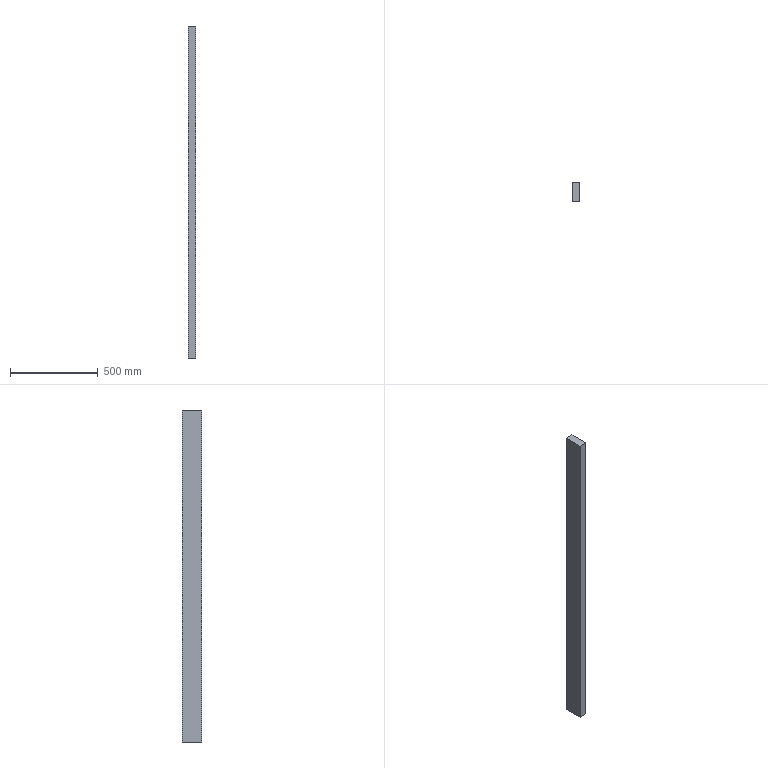Part | SolidWorks | features Extrusion 1 | 1 solid | 6 faces | box 45 x 110 x 1890 mm | volume 9355500 mm3 | plane 6
STEP:
#1=CARTESIAN_POINT('',(-22.5,55.,945.));
#2=VERTEX_POINT('',#1);
#3=CARTESIAN_POINT('',(-22.5,-55.,945.));
#4=VERTEX_POINT('',#3);
#5=CARTESIAN_POINT('',(-22.5,-55.,945.));
#6=DIRECTION('',(0.,-1.,0.));
#7=VECTOR('',#6,1000.);
#8=LINE('',#5,#7);
#9=EDGE_CURVE('',#2,#4,#8,.T.);
#10=ORIENTED_EDGE('',*,*,#9,.T.);
#11=CARTESIAN_POINT('',(22.5,-55.,945.));
#12=VERTEX_POINT('',#11);
#13=CARTESIAN_POINT('',(22.5,-55.,945.));
#14=DIRECTION('',(-1.,0.,0.));
#15=VECTOR('',#14,1000.);
#16=LINE('',#13,#15);
#17=EDGE_CURVE('',#12,#4,#16,.T.);
#18=ORIENTED_EDGE('',*,*,#17,.F.);
#19=CARTESIAN_POINT('',(22.5,55.,945.));
#20=VERTEX_POINT('',#19);
#21=CARTESIAN_POINT('',(22.5,-55.,945.));
#22=DIRECTION('',(0.,-1.,0.));
#23=VECTOR('',#22,1000.);
#24=LINE('',#21,#23);
#25=EDGE_CURVE('',#20,#12,#24,.T.);
#26=ORIENTED_EDGE('',*,*,#25,.F.);
#27=CARTESIAN_POINT('',(22.5,55.,945.));
#28=DIRECTION('',(-1.,0.,0.));
#29=VECTOR('',#28,1000.);
#30=LINE('',#27,#29);
#31=EDGE_CURVE('',#20,#2,#30,.T.);
#32=ORIENTED_EDGE('',*,*,#31,.T.);
#33=EDGE_LOOP('',(#10,#18,#26,#32));
#34=FACE_OUTER_BOUND('',#33,.T.);
#35=CARTESIAN_POINT('',(22.5,-55.,945.));
#36=DIRECTION('',(0.,0.,-1.));
#37=DIRECTION('',(-1.,0.,0.));
#38=AXIS2_PLACEMENT_3D('',#35,#36,#37);
#39=PLANE('',#38);
#40=ADVANCED_FACE('',(#34),#39,.F.);
#41=CARTESIAN_POINT('',(-22.5,-55.,-945.));
#42=VERTEX_POINT('',#41);
#43=CARTESIAN_POINT('',(-22.5,-55.,-945.));
#44=DIRECTION('',(0.,0.,-1.));
#45=VECTOR('',#44,1000.);
#46=LINE('',#43,#45);
#47=EDGE_CURVE('',#4,#42,#46,.T.);
#48=ORIENTED_EDGE('',*,*,#47,.T.);
#49=CARTESIAN_POINT('',(22.5,-55.,-945.));
#50=VERTEX_POINT('',#49);
#51=CARTESIAN_POINT('',(22.5,-55.,-945.));
#52=DIRECTION('',(-1.,0.,0.));
#53=VECTOR('',#52,1000.);
#54=LINE('',#51,#53);
#55=EDGE_CURVE('',#50,#42,#54,.T.);
#56=ORIENTED_EDGE('',*,*,#55,.F.);
#57=CARTESIAN_POINT('',(22.5,-55.,-945.));
#58=DIRECTION('',(0.,0.,-1.));
#59=VECTOR('',#58,1000.);
#60=LINE('',#57,#59);
#61=EDGE_CURVE('',#12,#50,#60,.T.);
#62=ORIENTED_EDGE('',*,*,#61,.F.);
#63=ORIENTED_EDGE('',*,*,#17,.T.);
#64=EDGE_LOOP('',(#48,#56,#62,#63));
#65=FACE_OUTER_BOUND('',#64,.T.);
#66=CARTESIAN_POINT('',(22.5,-55.,-945.));
#67=DIRECTION('',(0.,1.,0.));
#68=DIRECTION('',(0.,0.,1.));
#69=AXIS2_PLACEMENT_3D('',#66,#67,#68);
#70=PLANE('',#69);
#71=ADVANCED_FACE('',(#65),#70,.F.);
#72=CARTESIAN_POINT('',(-22.5,55.,-945.));
#73=VERTEX_POINT('',#72);
#74=CARTESIAN_POINT('',(-22.5,-55.,-945.));
#75=DIRECTION('',(0.,1.,0.));
#76=VECTOR('',#75,1000.);
#77=LINE('',#74,#76);
#78=EDGE_CURVE('',#42,#73,#77,.T.);
#79=ORIENTED_EDGE('',*,*,#78,.T.);
#80=CARTESIAN_POINT('',(22.5,55.,-945.));
#81=VERTEX_POINT('',#80);
#82=CARTESIAN_POINT('',(22.5,55.,-945.));
#83=DIRECTION('',(-1.,0.,0.));
#84=VECTOR('',#83,1000.);
#85=LINE('',#82,#84);
#86=EDGE_CURVE('',#81,#73,#85,.T.);
#87=ORIENTED_EDGE('',*,*,#86,.F.);
#88=CARTESIAN_POINT('',(22.5,-55.,-945.));
#89=DIRECTION('',(0.,1.,0.));
#90=VECTOR('',#89,1000.);
#91=LINE('',#88,#90);
#92=EDGE_CURVE('',#50,#81,#91,.T.);
#93=ORIENTED_EDGE('',*,*,#92,.F.);
#94=ORIENTED_EDGE('',*,*,#55,.T.);
#95=EDGE_LOOP('',(#79,#87,#93,#94));
#96=FACE_OUTER_BOUND('',#95,.T.);
#97=CARTESIAN_POINT('',(22.5,-55.,-945.));
#98=DIRECTION('',(0.,0.,1.));
#99=DIRECTION('',(1.,0.,0.));
#100=AXIS2_PLACEMENT_3D('',#97,#98,#99);
#101=PLANE('',#100);
#102=ADVANCED_FACE('',(#96),#101,.F.);
#103=CARTESIAN_POINT('',(-22.5,55.,-945.));
#104=DIRECTION('',(0.,0.,1.));
#105=VECTOR('',#104,1000.);
#106=LINE('',#103,#105);
#107=EDGE_CURVE('',#73,#2,#106,.T.);
#108=ORIENTED_EDGE('',*,*,#107,.T.);
#109=ORIENTED_EDGE('',*,*,#31,.F.);
#110=CARTESIAN_POINT('',(22.5,55.,-945.));
#111=DIRECTION('',(0.,0.,1.));
#112=VECTOR('',#111,1000.);
#113=LINE('',#110,#112);
#114=EDGE_CURVE('',#81,#20,#113,.T.);
#115=ORIENTED_EDGE('',*,*,#114,.F.);
#116=ORIENTED_EDGE('',*,*,#86,.T.);
#117=EDGE_LOOP('',(#108,#109,#115,#116));
#118=FACE_OUTER_BOUND('',#117,.T.);
#119=CARTESIAN_POINT('',(22.5,55.,-945.));
#120=DIRECTION('',(0.,-1.,0.));
#121=DIRECTION('',(0.,0.,-1.));
#122=AXIS2_PLACEMENT_3D('',#119,#120,#121);
#123=PLANE('',#122);
#124=ADVANCED_FACE('',(#118),#123,.F.);
#125=ORIENTED_EDGE('',*,*,#25,.T.);
#126=ORIENTED_EDGE('',*,*,#61,.T.);
#127=ORIENTED_EDGE('',*,*,#92,.T.);
#128=ORIENTED_EDGE('',*,*,#114,.T.);
#129=EDGE_LOOP('',(#125,#126,#127,#128));
#130=FACE_OUTER_BOUND('',#129,.T.);
#131=CARTESIAN_POINT('',(22.5,0.,0.));
#132=DIRECTION('',(1.,0.,0.));
#133=DIRECTION('',(0.,0.,-1.));
#134=AXIS2_PLACEMENT_3D('',#131,#132,#133);
#135=PLANE('',#134);
#136=ADVANCED_FACE('',(#130),#135,.T.);
#137=ORIENTED_EDGE('',*,*,#9,.F.);
#138=ORIENTED_EDGE('',*,*,#107,.F.);
#139=ORIENTED_EDGE('',*,*,#78,.F.);
#140=ORIENTED_EDGE('',*,*,#47,.F.);
#141=EDGE_LOOP('',(#137,#138,#139,#140));
#142=FACE_OUTER_BOUND('',#141,.T.);
#143=CARTESIAN_POINT('',(-22.5,0.,0.));
#144=DIRECTION('',(1.,0.,0.));
#145=DIRECTION('',(0.,0.,-1.));
#146=AXIS2_PLACEMENT_3D('',#143,#144,#145);
#147=PLANE('',#146);
#148=ADVANCED_FACE('',(#142),#147,.F.);
#149=CLOSED_SHELL('',(#40,#71,#102,#124,#136,#148));
#150=MANIFOLD_SOLID_BREP('',#149);
#151=CARTESIAN_POINT('',(0.,0.,0.));
#152=DIRECTION('',(0.,0.,1.));
#153=DIRECTION('',(1.,0.,0.));
#154=AXIS2_PLACEMENT_3D('',#151,#152,#153);
#155=(LENGTH_UNIT()NAMED_UNIT(*)SI_UNIT(.MILLI.,.METRE.));
#156=UNCERTAINTY_MEASURE_WITH_UNIT(LENGTH_MEASURE(0.00001),#155,'','');
#157=(NAMED_UNIT(*)PLANE_ANGLE_UNIT()SI_UNIT($,.RADIAN.));
#158=(NAMED_UNIT(*)SI_UNIT($,.STERADIAN.)SOLID_ANGLE_UNIT());
#159=(GEOMETRIC_REPRESENTATION_CONTEXT(3)GLOBAL_UNCERTAINTY_ASSIGNED_CONTEXT((#156))GLOBAL_UNIT_ASSIGNED_CONTEXT((#155,#157,#158))REPRESENTATION_CONTEXT('',''));
#160=ADVANCED_BREP_SHAPE_REPRESENTATION('',(#150,#154),#159);